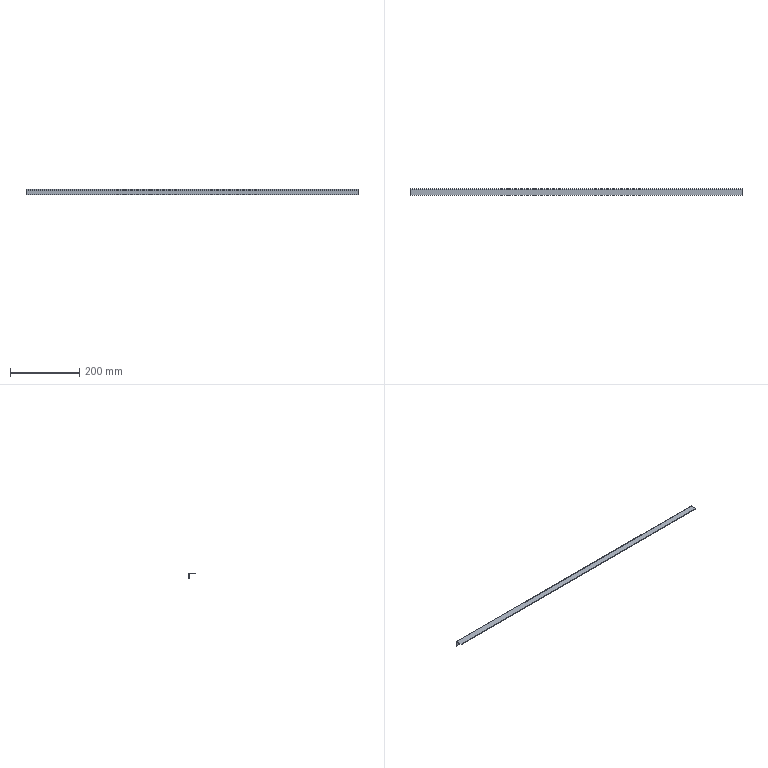Part | STEP file | Rear Closing Plate Door Frame Lower 1 | 1 solid | 10 faces | box 959 x 20 x 16 mm | volume 63977 mm3 | plane 8 | cylinder 2 | commonest cylinder face diameters 1 x1 5 x1
STEP:
#1=CARTESIAN_POINT('',(959.,-20.,16.));
#2=VERTEX_POINT('',#1);
#3=CARTESIAN_POINT('',(0.,-20.,16.));
#4=VERTEX_POINT('',#3);
#5=CARTESIAN_POINT('',(959.,-20.,16.));
#6=DIRECTION('',(-1.,0.,0.));
#7=VECTOR('',#6,1000.);
#8=LINE('',#5,#7);
#9=EDGE_CURVE('',#2,#4,#8,.T.);
#10=ORIENTED_EDGE('',*,*,#9,.F.);
#11=CARTESIAN_POINT('',(959.,-2.5,16.));
#12=VERTEX_POINT('',#11);
#13=CARTESIAN_POINT('',(959.,0.,16.));
#14=DIRECTION('',(0.,-1.,0.));
#15=VECTOR('',#14,1000.);
#16=LINE('',#13,#15);
#17=EDGE_CURVE('',#12,#2,#16,.T.);
#18=ORIENTED_EDGE('',*,*,#17,.F.);
#19=CARTESIAN_POINT('',(0.,-2.5,16.));
#20=VERTEX_POINT('',#19);
#21=CARTESIAN_POINT('',(959.,-2.5,16.));
#22=DIRECTION('',(1.,0.,0.));
#23=VECTOR('',#22,1000.);
#24=LINE('',#21,#23);
#25=EDGE_CURVE('',#20,#12,#24,.T.);
#26=ORIENTED_EDGE('',*,*,#25,.F.);
#27=CARTESIAN_POINT('',(0.,0.,16.));
#28=DIRECTION('',(0.,1.,0.));
#29=VECTOR('',#28,1000.);
#30=LINE('',#27,#29);
#31=EDGE_CURVE('',#4,#20,#30,.T.);
#32=ORIENTED_EDGE('',*,*,#31,.F.);
#33=EDGE_LOOP('',(#10,#18,#26,#32));
#34=FACE_OUTER_BOUND('',#33,.T.);
#35=CARTESIAN_POINT('',(959.,0.,16.));
#36=DIRECTION('',(0.,0.,-1.));
#37=DIRECTION('',(-1.,0.,0.));
#38=AXIS2_PLACEMENT_3D('',#35,#36,#37);
#39=PLANE('',#38);
#40=ADVANCED_FACE('',(#34),#39,.F.);
#41=CARTESIAN_POINT('',(0.,-2.5,14.));
#42=VERTEX_POINT('',#41);
#43=CARTESIAN_POINT('',(0.,-20.,14.));
#44=VERTEX_POINT('',#43);
#45=CARTESIAN_POINT('',(0.,-2.,14.));
#46=DIRECTION('',(0.,-1.,0.));
#47=VECTOR('',#46,1000.);
#48=LINE('',#45,#47);
#49=EDGE_CURVE('',#42,#44,#48,.T.);
#50=ORIENTED_EDGE('',*,*,#49,.T.);
#51=CARTESIAN_POINT('',(0.,-20.,13.5));
#52=DIRECTION('',(0.,0.,1.));
#53=VECTOR('',#52,1000.);
#54=LINE('',#51,#53);
#55=EDGE_CURVE('',#44,#4,#54,.T.);
#56=ORIENTED_EDGE('',*,*,#55,.T.);
#57=ORIENTED_EDGE('',*,*,#31,.T.);
#58=CARTESIAN_POINT('',(0.,0.,13.5));
#59=VERTEX_POINT('',#58);
#60=CARTESIAN_POINT('',(0.,-2.5,13.5));
#61=DIRECTION('',(1.,0.,0.));
#62=DIRECTION('',(0.,0.,1.));
#63=AXIS2_PLACEMENT_3D('',#60,#61,#62);
#64=CIRCLE('',#63,2.5);
#65=EDGE_CURVE('',#59,#20,#64,.T.);
#66=ORIENTED_EDGE('',*,*,#65,.F.);
#67=CARTESIAN_POINT('',(0.,0.,0.));
#68=VERTEX_POINT('',#67);
#69=CARTESIAN_POINT('',(0.,0.,0.));
#70=DIRECTION('',(0.,0.,-1.));
#71=VECTOR('',#70,1000.);
#72=LINE('',#69,#71);
#73=EDGE_CURVE('',#59,#68,#72,.T.);
#74=ORIENTED_EDGE('',*,*,#73,.T.);
#75=CARTESIAN_POINT('',(0.,-2.,0.));
#76=VERTEX_POINT('',#75);
#77=CARTESIAN_POINT('',(0.,-2.5,0.));
#78=DIRECTION('',(0.,1.,0.));
#79=VECTOR('',#78,1000.);
#80=LINE('',#77,#79);
#81=EDGE_CURVE('',#76,#68,#80,.T.);
#82=ORIENTED_EDGE('',*,*,#81,.F.);
#83=CARTESIAN_POINT('',(0.,-2.,13.5));
#84=VERTEX_POINT('',#83);
#85=CARTESIAN_POINT('',(0.,-2.,13.5));
#86=DIRECTION('',(0.,0.,-1.));
#87=VECTOR('',#86,1000.);
#88=LINE('',#85,#87);
#89=EDGE_CURVE('',#84,#76,#88,.T.);
#90=ORIENTED_EDGE('',*,*,#89,.F.);
#91=CARTESIAN_POINT('',(0.,-2.5,13.5));
#92=DIRECTION('',(1.,0.,0.));
#93=DIRECTION('',(0.,0.,1.));
#94=AXIS2_PLACEMENT_3D('',#91,#92,#93);
#95=CIRCLE('',#94,0.5);
#96=EDGE_CURVE('',#84,#42,#95,.T.);
#97=ORIENTED_EDGE('',*,*,#96,.T.);
#98=EDGE_LOOP('',(#50,#56,#57,#66,#74,#82,#90,#97));
#99=FACE_OUTER_BOUND('',#98,.T.);
#100=CARTESIAN_POINT('',(0.,-2.,13.5));
#101=DIRECTION('',(-1.,0.,0.));
#102=DIRECTION('',(0.,0.,1.));
#103=AXIS2_PLACEMENT_3D('',#100,#101,#102);
#104=PLANE('',#103);
#105=ADVANCED_FACE('',(#99),#104,.T.);
#106=CARTESIAN_POINT('',(959.,-20.,14.));
#107=VERTEX_POINT('',#106);
#108=CARTESIAN_POINT('',(959.,-20.,14.));
#109=DIRECTION('',(0.,0.,1.));
#110=VECTOR('',#109,1000.);
#111=LINE('',#108,#110);
#112=EDGE_CURVE('',#107,#2,#111,.T.);
#113=ORIENTED_EDGE('',*,*,#112,.T.);
#114=ORIENTED_EDGE('',*,*,#9,.T.);
#115=ORIENTED_EDGE('',*,*,#55,.F.);
#116=CARTESIAN_POINT('',(959.,-20.,14.));
#117=DIRECTION('',(1.,0.,0.));
#118=VECTOR('',#117,1000.);
#119=LINE('',#116,#118);
#120=EDGE_CURVE('',#44,#107,#119,.T.);
#121=ORIENTED_EDGE('',*,*,#120,.T.);
#122=EDGE_LOOP('',(#113,#114,#115,#121));
#123=FACE_OUTER_BOUND('',#122,.T.);
#124=CARTESIAN_POINT('',(959.,-20.,14.));
#125=DIRECTION('',(0.,-1.,0.));
#126=DIRECTION('',(0.,0.,-1.));
#127=AXIS2_PLACEMENT_3D('',#124,#125,#126);
#128=PLANE('',#127);
#129=ADVANCED_FACE('',(#123),#128,.T.);
#130=CARTESIAN_POINT('',(959.,-2.5,14.));
#131=VERTEX_POINT('',#130);
#132=CARTESIAN_POINT('',(959.,-2.5,14.));
#133=DIRECTION('',(0.,1.,0.));
#134=VECTOR('',#133,1000.);
#135=LINE('',#132,#134);
#136=EDGE_CURVE('',#107,#131,#135,.T.);
#137=ORIENTED_EDGE('',*,*,#136,.T.);
#138=CARTESIAN_POINT('',(959.,-2.,13.5));
#139=VERTEX_POINT('',#138);
#140=CARTESIAN_POINT('',(959.,-2.5,13.5));
#141=DIRECTION('',(-1.,0.,0.));
#142=DIRECTION('',(0.,0.,1.));
#143=AXIS2_PLACEMENT_3D('',#140,#141,#142);
#144=CIRCLE('',#143,0.5);
#145=EDGE_CURVE('',#131,#139,#144,.T.);
#146=ORIENTED_EDGE('',*,*,#145,.T.);
#147=CARTESIAN_POINT('',(959.,-2.,0.));
#148=VERTEX_POINT('',#147);
#149=CARTESIAN_POINT('',(959.,-2.,14.));
#150=DIRECTION('',(0.,0.,-1.));
#151=VECTOR('',#150,1000.);
#152=LINE('',#149,#151);
#153=EDGE_CURVE('',#139,#148,#152,.T.);
#154=ORIENTED_EDGE('',*,*,#153,.T.);
#155=CARTESIAN_POINT('',(959.,0.,0.));
#156=VERTEX_POINT('',#155);
#157=CARTESIAN_POINT('',(959.,-2.5,0.));
#158=DIRECTION('',(0.,1.,0.));
#159=VECTOR('',#158,1000.);
#160=LINE('',#157,#159);
#161=EDGE_CURVE('',#148,#156,#160,.T.);
#162=ORIENTED_EDGE('',*,*,#161,.T.);
#163=CARTESIAN_POINT('',(959.,0.,13.5));
#164=VERTEX_POINT('',#163);
#165=CARTESIAN_POINT('',(959.,0.,0.));
#166=DIRECTION('',(0.,0.,1.));
#167=VECTOR('',#166,1000.);
#168=LINE('',#165,#167);
#169=EDGE_CURVE('',#156,#164,#168,.T.);
#170=ORIENTED_EDGE('',*,*,#169,.T.);
#171=CARTESIAN_POINT('',(959.,-2.5,13.5));
#172=DIRECTION('',(-1.,0.,0.));
#173=DIRECTION('',(0.,0.,1.));
#174=AXIS2_PLACEMENT_3D('',#171,#172,#173);
#175=CIRCLE('',#174,2.5);
#176=EDGE_CURVE('',#12,#164,#175,.T.);
#177=ORIENTED_EDGE('',*,*,#176,.F.);
#178=ORIENTED_EDGE('',*,*,#17,.T.);
#179=ORIENTED_EDGE('',*,*,#112,.F.);
#180=EDGE_LOOP('',(#137,#146,#154,#162,#170,#177,#178,#179));
#181=FACE_OUTER_BOUND('',#180,.T.);
#182=CARTESIAN_POINT('',(959.,-2.5,13.5));
#183=DIRECTION('',(1.,0.,0.));
#184=DIRECTION('',(0.,0.,-1.));
#185=AXIS2_PLACEMENT_3D('',#182,#183,#184);
#186=PLANE('',#185);
#187=ADVANCED_FACE('',(#181),#186,.T.);
#188=ORIENTED_EDGE('',*,*,#176,.T.);
#189=CARTESIAN_POINT('',(959.,0.,13.5));
#190=DIRECTION('',(-1.,0.,0.));
#191=VECTOR('',#190,1000.);
#192=LINE('',#189,#191);
#193=EDGE_CURVE('',#164,#59,#192,.T.);
#194=ORIENTED_EDGE('',*,*,#193,.T.);
#195=ORIENTED_EDGE('',*,*,#65,.T.);
#196=ORIENTED_EDGE('',*,*,#25,.T.);
#197=EDGE_LOOP('',(#188,#194,#195,#196));
#198=FACE_OUTER_BOUND('',#197,.T.);
#199=CARTESIAN_POINT('',(959.,-2.5,13.5));
#200=DIRECTION('',(-1.,0.,0.));
#201=DIRECTION('',(0.,0.,1.));
#202=AXIS2_PLACEMENT_3D('',#199,#200,#201);
#203=CYLINDRICAL_SURFACE('',#202,2.5);
#204=ADVANCED_FACE('',(#198),#203,.T.);
#205=ORIENTED_EDGE('',*,*,#136,.F.);
#206=ORIENTED_EDGE('',*,*,#120,.F.);
#207=ORIENTED_EDGE('',*,*,#49,.F.);
#208=CARTESIAN_POINT('',(959.,-2.5,14.));
#209=DIRECTION('',(1.,0.,0.));
#210=VECTOR('',#209,1000.);
#211=LINE('',#208,#210);
#212=EDGE_CURVE('',#42,#131,#211,.T.);
#213=ORIENTED_EDGE('',*,*,#212,.T.);
#214=EDGE_LOOP('',(#205,#206,#207,#213));
#215=FACE_OUTER_BOUND('',#214,.T.);
#216=CARTESIAN_POINT('',(959.,0.,14.));
#217=DIRECTION('',(0.,0.,-1.));
#218=DIRECTION('',(-1.,0.,0.));
#219=AXIS2_PLACEMENT_3D('',#216,#217,#218);
#220=PLANE('',#219);
#221=ADVANCED_FACE('',(#215),#220,.T.);
#222=ORIENTED_EDGE('',*,*,#193,.F.);
#223=ORIENTED_EDGE('',*,*,#169,.F.);
#224=CARTESIAN_POINT('',(959.,0.,0.));
#225=DIRECTION('',(1.,0.,0.));
#226=VECTOR('',#225,1000.);
#227=LINE('',#224,#226);
#228=EDGE_CURVE('',#68,#156,#227,.T.);
#229=ORIENTED_EDGE('',*,*,#228,.F.);
#230=ORIENTED_EDGE('',*,*,#73,.F.);
#231=EDGE_LOOP('',(#222,#223,#229,#230));
#232=FACE_OUTER_BOUND('',#231,.T.);
#233=CARTESIAN_POINT('',(959.,0.,0.));
#234=DIRECTION('',(0.,-1.,0.));
#235=DIRECTION('',(0.,0.,-1.));
#236=AXIS2_PLACEMENT_3D('',#233,#234,#235);
#237=PLANE('',#236);
#238=ADVANCED_FACE('',(#232),#237,.F.);
#239=CARTESIAN_POINT('',(959.,-2.,13.5));
#240=DIRECTION('',(-1.,0.,0.));
#241=VECTOR('',#240,1000.);
#242=LINE('',#239,#241);
#243=EDGE_CURVE('',#139,#84,#242,.T.);
#244=ORIENTED_EDGE('',*,*,#243,.F.);
#245=ORIENTED_EDGE('',*,*,#145,.F.);
#246=ORIENTED_EDGE('',*,*,#212,.F.);
#247=ORIENTED_EDGE('',*,*,#96,.F.);
#248=EDGE_LOOP('',(#244,#245,#246,#247));
#249=FACE_OUTER_BOUND('',#248,.T.);
#250=CARTESIAN_POINT('',(959.,-2.5,13.5));
#251=DIRECTION('',(-1.,0.,0.));
#252=DIRECTION('',(0.,0.,1.));
#253=AXIS2_PLACEMENT_3D('',#250,#251,#252);
#254=CYLINDRICAL_SURFACE('',#253,0.5);
#255=ADVANCED_FACE('',(#249),#254,.F.);
#256=ORIENTED_EDGE('',*,*,#161,.F.);
#257=CARTESIAN_POINT('',(959.,-2.,0.));
#258=DIRECTION('',(-1.,0.,0.));
#259=VECTOR('',#258,1000.);
#260=LINE('',#257,#259);
#261=EDGE_CURVE('',#148,#76,#260,.T.);
#262=ORIENTED_EDGE('',*,*,#261,.T.);
#263=ORIENTED_EDGE('',*,*,#81,.T.);
#264=ORIENTED_EDGE('',*,*,#228,.T.);
#265=EDGE_LOOP('',(#256,#262,#263,#264));
#266=FACE_OUTER_BOUND('',#265,.T.);
#267=CARTESIAN_POINT('',(959.,0.,0.));
#268=DIRECTION('',(0.,0.,-1.));
#269=DIRECTION('',(0.,1.,0.));
#270=AXIS2_PLACEMENT_3D('',#267,#268,#269);
#271=PLANE('',#270);
#272=ADVANCED_FACE('',(#266),#271,.T.);
#273=ORIENTED_EDGE('',*,*,#153,.F.);
#274=ORIENTED_EDGE('',*,*,#243,.T.);
#275=ORIENTED_EDGE('',*,*,#89,.T.);
#276=ORIENTED_EDGE('',*,*,#261,.F.);
#277=EDGE_LOOP('',(#273,#274,#275,#276));
#278=FACE_OUTER_BOUND('',#277,.T.);
#279=CARTESIAN_POINT('',(959.,-2.,0.));
#280=DIRECTION('',(0.,-1.,0.));
#281=DIRECTION('',(0.,0.,-1.));
#282=AXIS2_PLACEMENT_3D('',#279,#280,#281);
#283=PLANE('',#282);
#284=ADVANCED_FACE('',(#278),#283,.T.);
#285=CLOSED_SHELL('',(#40,#105,#129,#187,#204,#221,#238,#255,#272,#284));
#286=MANIFOLD_SOLID_BREP('',#285);
#287=CARTESIAN_POINT('',(0.,0.,0.));
#288=DIRECTION('',(0.,0.,1.));
#289=DIRECTION('',(1.,0.,0.));
#290=AXIS2_PLACEMENT_3D('',#287,#288,#289);
#291=(LENGTH_UNIT()NAMED_UNIT(*)SI_UNIT(.MILLI.,.METRE.));
#292=UNCERTAINTY_MEASURE_WITH_UNIT(LENGTH_MEASURE(0.00001),#291,'','');
#293=(NAMED_UNIT(*)PLANE_ANGLE_UNIT()SI_UNIT($,.RADIAN.));
#294=(NAMED_UNIT(*)SI_UNIT($,.STERADIAN.)SOLID_ANGLE_UNIT());
#295=(GEOMETRIC_REPRESENTATION_CONTEXT(3)GLOBAL_UNCERTAINTY_ASSIGNED_CONTEXT((#292))GLOBAL_UNIT_ASSIGNED_CONTEXT((#291,#293,#294))REPRESENTATION_CONTEXT('',''));
#296=ADVANCED_BREP_SHAPE_REPRESENTATION('',(#286,#290),#295);